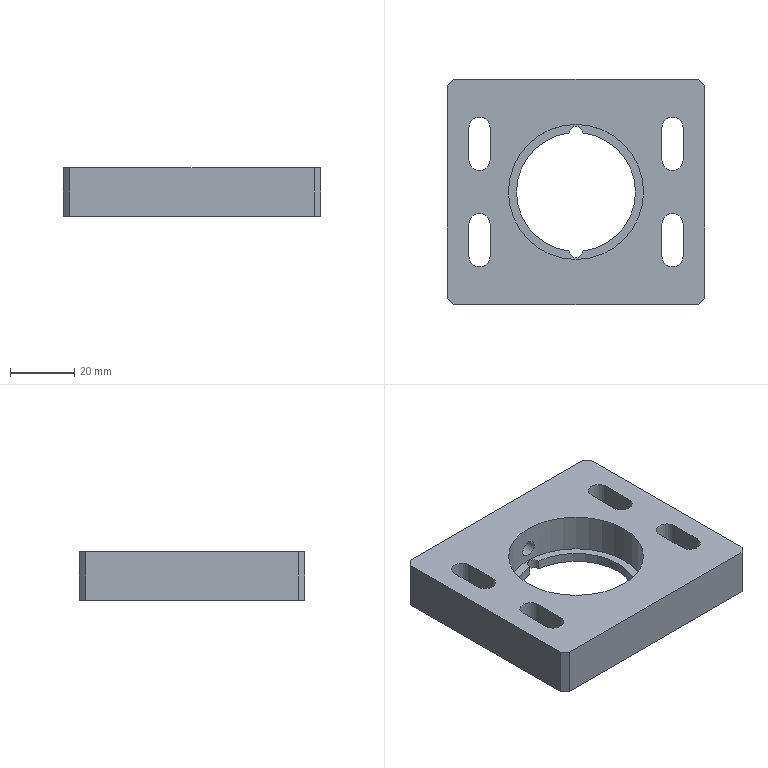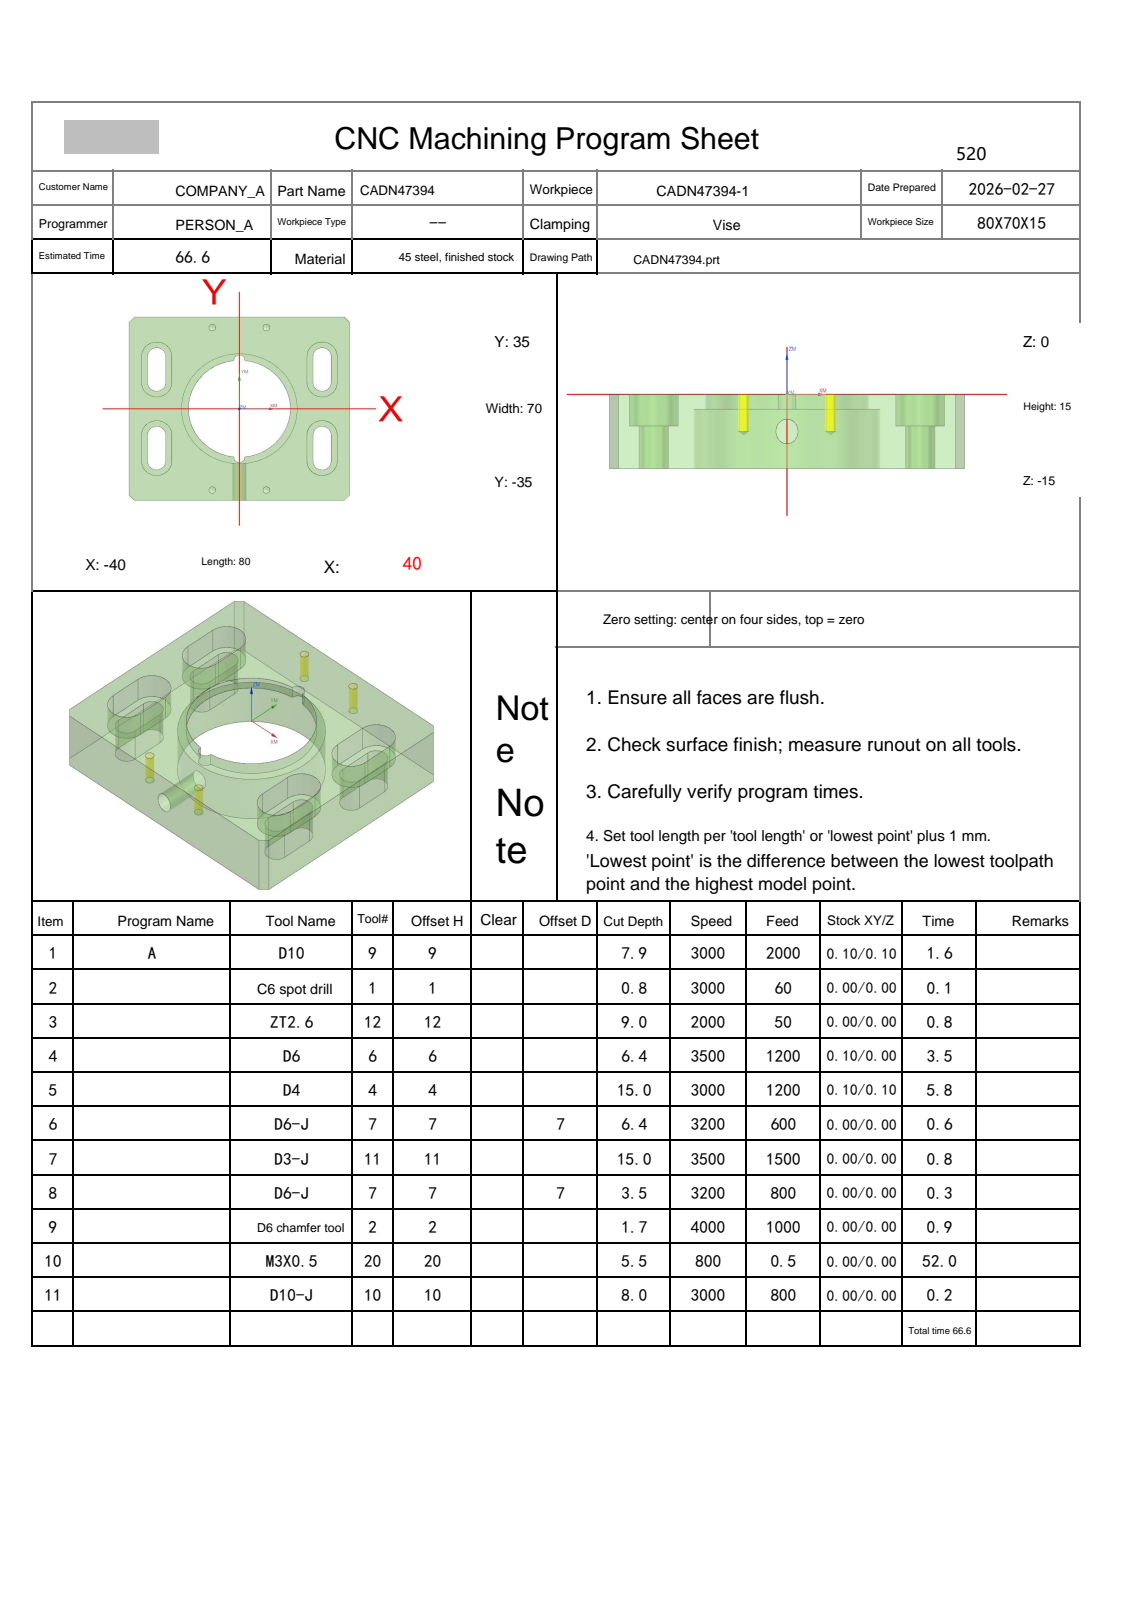NC program | NX | posted by the shop | part box 80 x 70 x 15 mm
Lines 1592 to 3269 of 4817, first 1205 of 1678 lines:
N5 T04 M06
(D4  D=4. R=0. H=04 ce=0.10 di=0.10)
G00 G90 G54 X31.2 Y15. M03 S3000
G43 H04 Z50.
M08
Z-5.9
G01 Y20. Z-5.927 F1200.
G03 X30. Y21.2 Z-5.937 I-1.2 J0.0
X28.8 Y20. Z-5.948 I0.0 J-1.2
G01 Y10. Z-6.002
G03 X30. Y8.8 Z-6.012 I1.2 J0.0
X31.2 Y10. Z-6.022 I0.0 J1.2
G01 Y20. Z-6.076
G03 X30. Y21.2 Z-6.086 I-1.2 J0.0
X28.8 Y20. Z-6.097 I0.0 J-1.2
G01 Y10. Z-6.151
G03 X30. Y8.8 Z-6.161 I1.2 J0.0
X31.2 Y10. Z-6.171 I0.0 J1.2
G01 Y20. Z-6.225
G03 X30. Y21.2 Z-6.236 I-1.2 J0.0
X28.8 Y20. Z-6.246 I0.0 J-1.2
G01 Y10. Z-6.3
G03 X30. Y8.8 Z-6.31 I1.2 J0.0
X31.2 Y10. Z-6.32 I0.0 J1.2
G01 Y20. Z-6.375
G03 X30. Y21.2 Z-6.385 I-1.2 J0.0
X28.8 Y20. Z-6.395 I0.0 J-1.2
G01 Y10. Z-6.449
G03 X30. Y8.8 Z-6.459 I1.2 J0.0
X31.2 Y10. Z-6.47 I0.0 J1.2
G01 Y20. Z-6.524
G03 X30. Y21.2 Z-6.534 I-1.2 J0.0
X28.8 Y20. Z-6.544 I0.0 J-1.2
G01 Y10. Z-6.598
G03 X30. Y8.8 Z-6.609 I1.2 J0.0
X31.2 Y10. Z-6.619 I0.0 J1.2
G01 Y20. Z-6.673
G03 X30. Y21.2 Z-6.683 I-1.2 J0.0
X28.8 Y20. Z-6.693 I0.0 J-1.2
G01 Y10. Z-6.748
G03 X30. Y8.8 Z-6.758 I1.2 J0.0
X31.2 Y10. Z-6.768 I0.0 J1.2
G01 Y20. Z-6.822
G03 X30. Y21.2 Z-6.832 I-1.2 J0.0
X28.8 Y20. Z-6.843 I0.0 J-1.2
G01 Y10. Z-6.897
G03 X30. Y8.8 Z-6.907 I1.2 J0.0
X31.2 Y10. Z-6.917 I0.0 J1.2
G01 Y20. Z-6.971
G03 X30. Y21.2 Z-6.982 I-1.2 J0.0
X28.8 Y20. Z-6.992 I0.0 J-1.2
G01 Y10. Z-7.046
G03 X30. Y8.8 Z-7.056 I1.2 J0.0
X31.2 Y10. Z-7.066 I0.0 J1.2
G01 Y20. Z-7.121
G03 X30. Y21.2 Z-7.131 I-1.2 J0.0
X28.8 Y20. Z-7.141 I0.0 J-1.2
G01 Y10. Z-7.195
G03 X30. Y8.8 Z-7.205 I1.2 J0.0
X31.2 Y10. Z-7.216 I0.0 J1.2
G01 Y20. Z-7.27
G03 X30. Y21.2 Z-7.28 I-1.2 J0.0
X28.8 Y20. Z-7.29 I0.0 J-1.2
G01 Y10. Z-7.344
G03 X30. Y8.8 Z-7.355 I1.2 J0.0
X31.2 Y10. Z-7.365 I0.0 J1.2
G01 Y20. Z-7.419
G03 X30. Y21.2 Z-7.429 I-1.2 J0.0
X28.8 Y20. Z-7.439 I0.0 J-1.2
G01 Y10. Z-7.493
G03 X30. Y8.8 Z-7.504 I1.2 J0.0
X31.2 Y10. Z-7.514 I0.0 J1.2
G01 Y20. Z-7.568
G03 X30. Y21.2 Z-7.578 I-1.2 J0.0
X28.8 Y20. Z-7.588 I0.0 J-1.2
G01 Y10. Z-7.643
G03 X30. Y8.8 Z-7.653 I1.2 J0.0
X31.2 Y10. Z-7.663 I0.0 J1.2
G01 Y20. Z-7.717
G03 X30. Y21.2 Z-7.727 I-1.2 J0.0
X28.8 Y20. Z-7.738 I0.0 J-1.2
G01 Y10. Z-7.792
G03 X30. Y8.8 Z-7.802 I1.2 J0.0
X31.2 Y10. Z-7.812 I0.0 J1.2
G01 Y20. Z-7.866
G03 X30. Y21.2 Z-7.877 I-1.2 J0.0
X28.8 Y20. Z-7.887 I0.0 J-1.2
G01 Y10. Z-7.941
G03 X30. Y8.8 Z-7.951 I1.2 J0.0
X31.2 Y10. Z-7.961 I0.0 J1.2
G01 Y20. Z-8.016
G03 X30. Y21.2 Z-8.026 I-1.2 J0.0
X28.8 Y20. Z-8.036 I0.0 J-1.2
G01 Y10. Z-8.09
G03 X30. Y8.8 Z-8.1 I1.2 J0.0
X31.2 Y10. Z-8.111 I0.0 J1.2
G01 Y20. Z-8.165
G03 X30. Y21.2 Z-8.175 I-1.2 J0.0
X28.8 Y20. Z-8.185 I0.0 J-1.2
G01 Y10. Z-8.239
G03 X30. Y8.8 Z-8.25 I1.2 J0.0
X31.2 Y10. Z-8.26 I0.0 J1.2
G01 Y20. Z-8.314
G03 X30. Y21.2 Z-8.324 I-1.2 J0.0
X28.8 Y20. Z-8.334 I0.0 J-1.2
G01 Y10. Z-8.389
G03 X30. Y8.8 Z-8.399 I1.2 J0.0
X31.2 Y10. Z-8.409 I0.0 J1.2
G01 Y20. Z-8.463
G03 X30. Y21.2 Z-8.473 I-1.2 J0.0
X28.8 Y20. Z-8.484 I0.0 J-1.2
G01 Y10. Z-8.538
G03 X30. Y8.8 Z-8.548 I1.2 J0.0
X31.2 Y10. Z-8.558 I0.0 J1.2
G01 Y20. Z-8.612
G03 X30. Y21.2 Z-8.623 I-1.2 J0.0
X28.8 Y20. Z-8.633 I0.0 J-1.2
G01 Y10. Z-8.687
G03 X30. Y8.8 Z-8.697 I1.2 J0.0
X31.2 Y10. Z-8.707 I0.0 J1.2
G01 Y20. Z-8.762
G03 X30. Y21.2 Z-8.772 I-1.2 J0.0
X28.8 Y20. Z-8.782 I0.0 J-1.2
G01 Y10. Z-8.836
G03 X30. Y8.8 Z-8.846 I1.2 J0.0
X31.2 Y10. Z-8.857 I0.0 J1.2
G01 Y20. Z-8.911
G03 X30. Y21.2 Z-8.921 I-1.2 J0.0
X28.8 Y20. Z-8.931 I0.0 J-1.2
G01 Y10. Z-8.985
G03 X30. Y8.8 Z-8.995 I1.2 J0.0
X31.2 Y10. Z-9.006 I0.0 J1.2
G01 Y20. Z-9.06
G03 X30. Y21.2 Z-9.07 I-1.2 J0.0
X28.8 Y20. Z-9.08 I0.0 J-1.2
G01 Y10. Z-9.134
G03 X30. Y8.8 Z-9.145 I1.2 J0.0
X31.2 Y10. Z-9.155 I0.0 J1.2
G01 Y20. Z-9.209
G03 X30. Y21.2 Z-9.219 I-1.2 J0.0
X28.8 Y20. Z-9.229 I0.0 J-1.2
G01 Y10. Z-9.284
G03 X30. Y8.8 Z-9.294 I1.2 J0.0
X31.2 Y10. Z-9.304 I0.0 J1.2
G01 Y20. Z-9.358
G03 X30. Y21.2 Z-9.368 I-1.2 J0.0
X28.8 Y20. Z-9.379 I0.0 J-1.2
G01 Y10. Z-9.433
G03 X30. Y8.8 Z-9.443 I1.2 J0.0
X31.2 Y10. Z-9.453 I0.0 J1.2
G01 Y20. Z-9.507
G03 X30. Y21.2 Z-9.518 I-1.2 J0.0
X28.8 Y20. Z-9.528 I0.0 J-1.2
G01 Y10. Z-9.582
G03 X30. Y8.8 Z-9.592 I1.2 J0.0
X31.2 Y10. Z-9.602 I0.0 J1.2
G01 Y20. Z-9.657
G03 X30. Y21.2 Z-9.667 I-1.2 J0.0
X28.8 Y20. Z-9.677 I0.0 J-1.2
G01 Y10. Z-9.731
G03 X30. Y8.8 Z-9.741 I1.2 J0.0
X31.2 Y10. Z-9.752 I0.0 J1.2
G01 Y20. Z-9.806
G03 X30. Y21.2 Z-9.816 I-1.2 J0.0
X28.8 Y20. Z-9.826 I0.0 J-1.2
G01 Y10. Z-9.88
G03 X30. Y8.8 Z-9.891 I1.2 J0.0
X31.2 Y10. Z-9.901 I0.0 J1.2
G01 Y20. Z-9.955
G03 X30. Y21.2 Z-9.965 I-1.2 J0.0
X28.8 Y20. Z-9.975 I0.0 J-1.2
G01 Y10. Z-10.03
G03 X30. Y8.8 Z-10.04 I1.2 J0.0
X31.2 Y10. Z-10.05 I0.0 J1.2
G01 Y20. Z-10.104
G03 X30. Y21.2 Z-10.114 I-1.2 J0.0
X28.8 Y20. Z-10.125 I0.0 J-1.2
G01 Y10. Z-10.179
G03 X30. Y8.8 Z-10.189 I1.2 J0.0
X31.2 Y10. Z-10.199 I0.0 J1.2
G01 Y20. Z-10.253
G03 X30. Y21.2 Z-10.264 I-1.2 J0.0
X28.8 Y20. Z-10.274 I0.0 J-1.2
G01 Y10. Z-10.328
G03 X30. Y8.8 Z-10.338 I1.2 J0.0
X31.2 Y10. Z-10.348 I0.0 J1.2
G01 Y20. Z-10.402
G03 X30. Y21.2 Z-10.413 I-1.2 J0.0
X28.8 Y20. Z-10.423 I0.0 J-1.2
G01 Y10. Z-10.477
G03 X30. Y8.8 Z-10.487 I1.2 J0.0
X31.2 Y10. Z-10.498 I0.0 J1.2
G01 Y20. Z-10.552
G03 X30. Y21.2 Z-10.562 I-1.2 J0.0
X28.8 Y20. Z-10.572 I0.0 J-1.2
G01 Y10. Z-10.626
G03 X30. Y8.8 Z-10.636 I1.2 J0.0
X31.2 Y10. Z-10.647 I0.0 J1.2
G01 Y20. Z-10.701
G03 X30. Y21.2 Z-10.711 I-1.2 J0.0
X28.8 Y20. Z-10.721 I0.0 J-1.2
G01 Y10. Z-10.775
G03 X30. Y8.8 Z-10.786 I1.2 J0.0
X31.2 Y10. Z-10.796 I0.0 J1.2
G01 Y20. Z-10.85
G03 X30. Y21.2 Z-10.86 I-1.2 J0.0
X28.8 Y20. Z-10.87 I0.0 J-1.2
G01 Y10. Z-10.925
G03 X30. Y8.8 Z-10.935 I1.2 J0.0
X31.2 Y10. Z-10.945 I0.0 J1.2
G01 Y20. Z-10.999
G03 X30. Y21.2 Z-11.009 I-1.2 J0.0
X28.8 Y20. Z-11.02 I0.0 J-1.2
G01 Y10. Z-11.074
G03 X30. Y8.8 Z-11.084 I1.2 J0.0
X31.2 Y10. Z-11.094 I0.0 J1.2
G01 Y20. Z-11.148
G03 X30. Y21.2 Z-11.159 I-1.2 J0.0
X28.8 Y20. Z-11.169 I0.0 J-1.2
G01 Y10. Z-11.223
G03 X30. Y8.8 Z-11.233 I1.2 J0.0
X31.2 Y10. Z-11.243 I0.0 J1.2
G01 Y20. Z-11.298
G03 X30. Y21.2 Z-11.308 I-1.2 J0.0
X28.8 Y20. Z-11.318 I0.0 J-1.2
G01 Y10. Z-11.372
G03 X30. Y8.8 Z-11.382 I1.2 J0.0
X31.2 Y10. Z-11.393 I0.0 J1.2
G01 Y20. Z-11.447
G03 X30. Y21.2 Z-11.457 I-1.2 J0.0
X28.8 Y20. Z-11.467 I0.0 J-1.2
G01 Y10. Z-11.521
G03 X30. Y8.8 Z-11.532 I1.2 J0.0
X31.2 Y10. Z-11.542 I0.0 J1.2
G01 Y20. Z-11.596
G03 X30. Y21.2 Z-11.606 I-1.2 J0.0
X28.8 Y20. Z-11.616 I0.0 J-1.2
G01 Y10. Z-11.671
G03 X30. Y8.8 Z-11.681 I1.2 J0.0
X31.2 Y10. Z-11.691 I0.0 J1.2
G01 Y20. Z-11.745
G03 X30. Y21.2 Z-11.755 I-1.2 J0.0
X28.8 Y20. Z-11.766 I0.0 J-1.2
G01 Y10. Z-11.82
G03 X30. Y8.8 Z-11.83 I1.2 J0.0
X31.2 Y10. Z-11.84 I0.0 J1.2
G01 Y20. Z-11.894
G03 X30. Y21.2 Z-11.905 I-1.2 J0.0
X28.8 Y20. Z-11.915 I0.0 J-1.2
G01 Y10. Z-11.969
G03 X30. Y8.8 Z-11.979 I1.2 J0.0
X31.2 Y10. Z-11.989 I0.0 J1.2
G01 Y20. Z-12.043
G03 X30. Y21.2 Z-12.054 I-1.2 J0.0
X28.8 Y20. Z-12.064 I0.0 J-1.2
G01 Y10. Z-12.118
G03 X30. Y8.8 Z-12.128 I1.2 J0.0
X31.2 Y10. Z-12.138 I0.0 J1.2
G01 Y20. Z-12.193
G03 X30. Y21.2 Z-12.203 I-1.2 J0.0
X28.8 Y20. Z-12.213 I0.0 J-1.2
G01 Y10. Z-12.267
G03 X30. Y8.8 Z-12.277 I1.2 J0.0
X31.2 Y10. Z-12.288 I0.0 J1.2
G01 Y20. Z-12.342
G03 X30. Y21.2 Z-12.352 I-1.2 J0.0
X28.8 Y20. Z-12.362 I0.0 J-1.2
G01 Y10. Z-12.416
G03 X30. Y8.8 Z-12.427 I1.2 J0.0
X31.2 Y10. Z-12.437 I0.0 J1.2
G01 Y20. Z-12.491
G03 X30. Y21.2 Z-12.501 I-1.2 J0.0
X28.8 Y20. Z-12.511 I0.0 J-1.2
G01 Y10. Z-12.566
G03 X30. Y8.8 Z-12.576 I1.2 J0.0
X31.2 Y10. Z-12.586 I0.0 J1.2
G01 Y20. Z-12.64
G03 X30. Y21.2 Z-12.65 I-1.2 J0.0
X28.8 Y20. Z-12.661 I0.0 J-1.2
G01 Y10. Z-12.715
G03 X30. Y8.8 Z-12.725 I1.2 J0.0
X31.2 Y10. Z-12.735 I0.0 J1.2
G01 Y20. Z-12.789
G03 X30. Y21.2 Z-12.8 I-1.2 J0.0
X28.8 Y20. Z-12.81 I0.0 J-1.2
G01 Y10. Z-12.864
G03 X30. Y8.8 Z-12.874 I1.2 J0.0
X31.2 Y10. Z-12.884 I0.0 J1.2
G01 Y20. Z-12.939
G03 X30. Y21.2 Z-12.949 I-1.2 J0.0
X28.8 Y20. Z-12.959 I0.0 J-1.2
G01 Y10. Z-13.013
G03 X30. Y8.8 Z-13.023 I1.2 J0.0
X31.2 Y10. Z-13.034 I0.0 J1.2
G01 Y20. Z-13.088
G03 X30. Y21.2 Z-13.098 I-1.2 J0.0
X28.8 Y20. Z-13.108 I0.0 J-1.2
G01 Y10. Z-13.162
G03 X30. Y8.8 Z-13.173 I1.2 J0.0
X31.2 Y10. Z-13.183 I0.0 J1.2
G01 Y20. Z-13.237
G03 X30. Y21.2 Z-13.247 I-1.2 J0.0
X28.8 Y20. Z-13.257 I0.0 J-1.2
G01 Y10. Z-13.312
G03 X30. Y8.8 Z-13.322 I1.2 J0.0
X31.2 Y10. Z-13.332 I0.0 J1.2
G01 Y20. Z-13.386
G03 X30. Y21.2 Z-13.396 I-1.2 J0.0
X28.8 Y20. Z-13.407 I0.0 J-1.2
G01 Y10. Z-13.461
G03 X30. Y8.8 Z-13.471 I1.2 J0.0
X31.2 Y10. Z-13.481 I0.0 J1.2
G01 Y20. Z-13.535
G03 X30. Y21.2 Z-13.545 I-1.2 J0.0
X28.8 Y20. Z-13.556 I0.0 J-1.2
G01 Y10. Z-13.61
G03 X30. Y8.8 Z-13.62 I1.2 J0.0
X31.2 Y10. Z-13.63 I0.0 J1.2
G01 Y20. Z-13.684
G03 X30. Y21.2 Z-13.695 I-1.2 J0.0
X28.8 Y20. Z-13.705 I0.0 J-1.2
G01 Y10. Z-13.759
G03 X30. Y8.8 Z-13.769 I1.2 J0.0
X31.2 Y10. Z-13.779 I0.0 J1.2
G01 Y20. Z-13.834
G03 X30. Y21.2 Z-13.844 I-1.2 J0.0
X28.8 Y20. Z-13.854 I0.0 J-1.2
G01 Y10. Z-13.908
G03 X30. Y8.8 Z-13.918 I1.2 J0.0
X31.2 Y10. Z-13.929 I0.0 J1.2
G01 Y20. Z-13.983
G03 X30. Y21.2 Z-13.993 I-1.2 J0.0
X28.8 Y20. Z-14.003 I0.0 J-1.2
G01 Y10. Z-14.057
G03 X30. Y8.8 Z-14.068 I1.2 J0.0
X31.2 Y10. Z-14.078 I0.0 J1.2
G01 Y20. Z-14.132
G03 X30. Y21.2 Z-14.142 I-1.2 J0.0
X28.8 Y20. Z-14.152 I0.0 J-1.2
G01 Y10. Z-14.207
G03 X30. Y8.8 Z-14.217 I1.2 J0.0
X31.2 Y10. Z-14.227 I0.0 J1.2
G01 Y20. Z-14.281
G03 X30. Y21.2 Z-14.291 I-1.2 J0.0
X28.8 Y20. Z-14.302 I0.0 J-1.2
G01 Y10. Z-14.356
G03 X30. Y8.8 Z-14.366 I1.2 J0.0
X31.2 Y10. Z-14.376 I0.0 J1.2
G01 Y20. Z-14.43
G03 X30. Y21.2 Z-14.441 I-1.2 J0.0
X28.8 Y20. Z-14.451 I0.0 J-1.2
G01 Y10. Z-14.505
G03 X30. Y8.8 Z-14.515 I1.2 J0.0
X31.2 Y10. Z-14.525 I0.0 J1.2
G01 Y20. Z-14.58
G03 X30. Y21.2 Z-14.59 I-1.2 J0.0
X28.8 Y20. Z-14.6 I0.0 J-1.2
G01 Y10. Z-14.654
G03 X30. Y8.8 Z-14.664 I1.2 J0.0
X31.2 Y10. Z-14.675 I0.0 J1.2
G01 Y20. Z-14.729
G03 X30. Y21.2 Z-14.739 I-1.2 J0.0
X28.8 Y20. Z-14.749 I0.0 J-1.2
G01 Y10. Z-14.803
G03 X30. Y8.8 Z-14.814 I1.2 J0.0
X31.2 Y10. Z-14.824 I0.0 J1.2
G01 Y20. Z-14.878
G03 X30. Y21.2 Z-14.888 I-1.2 J0.0
X28.8 Y20. Z-14.898 I0.0 J-1.2
G01 Y10. Z-14.952
G03 X30. Y8.8 Z-14.963 I1.2 J0.0
X31.2 Y10. Z-14.973 I0.0 J1.2
G01 Y15. Z-15.
Y20.
G03 X30. Y21.2 I-1.2 J0.0
X28.8 Y20. I0.0 J-1.2
G01 Y10.
G03 X30. Y8.8 I1.2 J0.0
X31.2 Y10. I0.0 J1.2
G01 Y15.
Y15.5
Z-14.
G00 Z50.
Y-15.
Z-5.9
G01 Y-10. Z-5.927
G03 X30. Y-8.8 Z-5.937 I-1.2 J0.0
X28.8 Y-10. Z-5.948 I0.0 J-1.2
G01 Y-20. Z-6.002
G03 X30. Y-21.2 Z-6.012 I1.2 J0.0
X31.2 Y-20. Z-6.022 I0.0 J1.2
G01 Y-10. Z-6.076
G03 X30. Y-8.8 Z-6.086 I-1.2 J0.0
X28.8 Y-10. Z-6.097 I0.0 J-1.2
G01 Y-20. Z-6.151
G03 X30. Y-21.2 Z-6.161 I1.2 J0.0
X31.2 Y-20. Z-6.171 I0.0 J1.2
G01 Y-10. Z-6.225
G03 X30. Y-8.8 Z-6.236 I-1.2 J0.0
X28.8 Y-10. Z-6.246 I0.0 J-1.2
G01 Y-20. Z-6.3
G03 X30. Y-21.2 Z-6.31 I1.2 J0.0
X31.2 Y-20. Z-6.32 I0.0 J1.2
G01 Y-10. Z-6.375
G03 X30. Y-8.8 Z-6.385 I-1.2 J0.0
X28.8 Y-10. Z-6.395 I0.0 J-1.2
G01 Y-20. Z-6.449
G03 X30. Y-21.2 Z-6.459 I1.2 J0.0
X31.2 Y-20. Z-6.47 I0.0 J1.2
G01 Y-10. Z-6.524
G03 X30. Y-8.8 Z-6.534 I-1.2 J0.0
X28.8 Y-10. Z-6.544 I0.0 J-1.2
G01 Y-20. Z-6.598
G03 X30. Y-21.2 Z-6.609 I1.2 J0.0
X31.2 Y-20. Z-6.619 I0.0 J1.2
G01 Y-10. Z-6.673
G03 X30. Y-8.8 Z-6.683 I-1.2 J0.0
X28.8 Y-10. Z-6.693 I0.0 J-1.2
G01 Y-20. Z-6.748
G03 X30. Y-21.2 Z-6.758 I1.2 J0.0
X31.2 Y-20. Z-6.768 I0.0 J1.2
G01 Y-10. Z-6.822
G03 X30. Y-8.8 Z-6.832 I-1.2 J0.0
X28.8 Y-10. Z-6.843 I0.0 J-1.2
G01 Y-20. Z-6.897
G03 X30. Y-21.2 Z-6.907 I1.2 J0.0
X31.2 Y-20. Z-6.917 I0.0 J1.2
G01 Y-10. Z-6.971
G03 X30. Y-8.8 Z-6.982 I-1.2 J0.0
X28.8 Y-10. Z-6.992 I0.0 J-1.2
G01 Y-20. Z-7.046
G03 X30. Y-21.2 Z-7.056 I1.2 J0.0
X31.2 Y-20. Z-7.066 I0.0 J1.2
G01 Y-10. Z-7.121
G03 X30. Y-8.8 Z-7.131 I-1.2 J0.0
X28.8 Y-10. Z-7.141 I0.0 J-1.2
G01 Y-20. Z-7.195
G03 X30. Y-21.2 Z-7.205 I1.2 J0.0
X31.2 Y-20. Z-7.216 I0.0 J1.2
G01 Y-10. Z-7.27
G03 X30. Y-8.8 Z-7.28 I-1.2 J0.0
X28.8 Y-10. Z-7.29 I0.0 J-1.2
G01 Y-20. Z-7.344
G03 X30. Y-21.2 Z-7.355 I1.2 J0.0
X31.2 Y-20. Z-7.365 I0.0 J1.2
G01 Y-10. Z-7.419
G03 X30. Y-8.8 Z-7.429 I-1.2 J0.0
X28.8 Y-10. Z-7.439 I0.0 J-1.2
G01 Y-20. Z-7.493
G03 X30. Y-21.2 Z-7.504 I1.2 J0.0
X31.2 Y-20. Z-7.514 I0.0 J1.2
G01 Y-10. Z-7.568
G03 X30. Y-8.8 Z-7.578 I-1.2 J0.0
X28.8 Y-10. Z-7.588 I0.0 J-1.2
G01 Y-20. Z-7.643
G03 X30. Y-21.2 Z-7.653 I1.2 J0.0
X31.2 Y-20. Z-7.663 I0.0 J1.2
G01 Y-10. Z-7.717
G03 X30. Y-8.8 Z-7.727 I-1.2 J0.0
X28.8 Y-10. Z-7.738 I0.0 J-1.2
G01 Y-20. Z-7.792
G03 X30. Y-21.2 Z-7.802 I1.2 J0.0
X31.2 Y-20. Z-7.812 I0.0 J1.2
G01 Y-10. Z-7.866
G03 X30. Y-8.8 Z-7.877 I-1.2 J0.0
X28.8 Y-10. Z-7.887 I0.0 J-1.2
G01 Y-20. Z-7.941
G03 X30. Y-21.2 Z-7.951 I1.2 J0.0
X31.2 Y-20. Z-7.961 I0.0 J1.2
G01 Y-10. Z-8.016
G03 X30. Y-8.8 Z-8.026 I-1.2 J0.0
X28.8 Y-10. Z-8.036 I0.0 J-1.2
G01 Y-20. Z-8.09
G03 X30. Y-21.2 Z-8.1 I1.2 J0.0
X31.2 Y-20. Z-8.111 I0.0 J1.2
G01 Y-10. Z-8.165
G03 X30. Y-8.8 Z-8.175 I-1.2 J0.0
X28.8 Y-10. Z-8.185 I0.0 J-1.2
G01 Y-20. Z-8.239
G03 X30. Y-21.2 Z-8.25 I1.2 J0.0
X31.2 Y-20. Z-8.26 I0.0 J1.2
G01 Y-10. Z-8.314
G03 X30. Y-8.8 Z-8.324 I-1.2 J0.0
X28.8 Y-10. Z-8.334 I0.0 J-1.2
G01 Y-20. Z-8.389
G03 X30. Y-21.2 Z-8.399 I1.2 J0.0
X31.2 Y-20. Z-8.409 I0.0 J1.2
G01 Y-10. Z-8.463
G03 X30. Y-8.8 Z-8.473 I-1.2 J0.0
X28.8 Y-10. Z-8.484 I0.0 J-1.2
G01 Y-20. Z-8.538
G03 X30. Y-21.2 Z-8.548 I1.2 J0.0
X31.2 Y-20. Z-8.558 I0.0 J1.2
G01 Y-10. Z-8.612
G03 X30. Y-8.8 Z-8.623 I-1.2 J0.0
X28.8 Y-10. Z-8.633 I0.0 J-1.2
G01 Y-20. Z-8.687
G03 X30. Y-21.2 Z-8.697 I1.2 J0.0
X31.2 Y-20. Z-8.707 I0.0 J1.2
G01 Y-10. Z-8.762
G03 X30. Y-8.8 Z-8.772 I-1.2 J0.0
X28.8 Y-10. Z-8.782 I0.0 J-1.2
G01 Y-20. Z-8.836
G03 X30. Y-21.2 Z-8.846 I1.2 J0.0
X31.2 Y-20. Z-8.857 I0.0 J1.2
G01 Y-10. Z-8.911
G03 X30. Y-8.8 Z-8.921 I-1.2 J0.0
X28.8 Y-10. Z-8.931 I0.0 J-1.2
G01 Y-20. Z-8.985
G03 X30. Y-21.2 Z-8.995 I1.2 J0.0
X31.2 Y-20. Z-9.006 I0.0 J1.2
G01 Y-10. Z-9.06
G03 X30. Y-8.8 Z-9.07 I-1.2 J0.0
X28.8 Y-10. Z-9.08 I0.0 J-1.2
G01 Y-20. Z-9.134
G03 X30. Y-21.2 Z-9.145 I1.2 J0.0
X31.2 Y-20. Z-9.155 I0.0 J1.2
G01 Y-10. Z-9.209
G03 X30. Y-8.8 Z-9.219 I-1.2 J0.0
X28.8 Y-10. Z-9.229 I0.0 J-1.2
G01 Y-20. Z-9.284
G03 X30. Y-21.2 Z-9.294 I1.2 J0.0
X31.2 Y-20. Z-9.304 I0.0 J1.2
G01 Y-10. Z-9.358
G03 X30. Y-8.8 Z-9.368 I-1.2 J0.0
X28.8 Y-10. Z-9.379 I0.0 J-1.2
G01 Y-20. Z-9.433
G03 X30. Y-21.2 Z-9.443 I1.2 J0.0
X31.2 Y-20. Z-9.453 I0.0 J1.2
G01 Y-10. Z-9.507
G03 X30. Y-8.8 Z-9.518 I-1.2 J0.0
X28.8 Y-10. Z-9.528 I0.0 J-1.2
G01 Y-20. Z-9.582
G03 X30. Y-21.2 Z-9.592 I1.2 J0.0
X31.2 Y-20. Z-9.602 I0.0 J1.2
G01 Y-10. Z-9.657
G03 X30. Y-8.8 Z-9.667 I-1.2 J0.0
X28.8 Y-10. Z-9.677 I0.0 J-1.2
G01 Y-20. Z-9.731
G03 X30. Y-21.2 Z-9.741 I1.2 J0.0
X31.2 Y-20. Z-9.752 I0.0 J1.2
G01 Y-10. Z-9.806
G03 X30. Y-8.8 Z-9.816 I-1.2 J0.0
X28.8 Y-10. Z-9.826 I0.0 J-1.2
G01 Y-20. Z-9.88
G03 X30. Y-21.2 Z-9.891 I1.2 J0.0
X31.2 Y-20. Z-9.901 I0.0 J1.2
G01 Y-10. Z-9.955
G03 X30. Y-8.8 Z-9.965 I-1.2 J0.0
X28.8 Y-10. Z-9.975 I0.0 J-1.2
G01 Y-20. Z-10.03
G03 X30. Y-21.2 Z-10.04 I1.2 J0.0
X31.2 Y-20. Z-10.05 I0.0 J1.2
G01 Y-10. Z-10.104
G03 X30. Y-8.8 Z-10.114 I-1.2 J0.0
X28.8 Y-10. Z-10.125 I0.0 J-1.2
G01 Y-20. Z-10.179
G03 X30. Y-21.2 Z-10.189 I1.2 J0.0
X31.2 Y-20. Z-10.199 I0.0 J1.2
G01 Y-10. Z-10.253
G03 X30. Y-8.8 Z-10.264 I-1.2 J0.0
X28.8 Y-10. Z-10.274 I0.0 J-1.2
G01 Y-20. Z-10.328
G03 X30. Y-21.2 Z-10.338 I1.2 J0.0
X31.2 Y-20. Z-10.348 I0.0 J1.2
G01 Y-10. Z-10.402
G03 X30. Y-8.8 Z-10.413 I-1.2 J0.0
X28.8 Y-10. Z-10.423 I0.0 J-1.2
G01 Y-20. Z-10.477
G03 X30. Y-21.2 Z-10.487 I1.2 J0.0
X31.2 Y-20. Z-10.498 I0.0 J1.2
G01 Y-10. Z-10.552
G03 X30. Y-8.8 Z-10.562 I-1.2 J0.0
X28.8 Y-10. Z-10.572 I0.0 J-1.2
G01 Y-20. Z-10.626
G03 X30. Y-21.2 Z-10.636 I1.2 J0.0
X31.2 Y-20. Z-10.647 I0.0 J1.2
G01 Y-10. Z-10.701
G03 X30. Y-8.8 Z-10.711 I-1.2 J0.0
X28.8 Y-10. Z-10.721 I0.0 J-1.2
G01 Y-20. Z-10.775
G03 X30. Y-21.2 Z-10.786 I1.2 J0.0
X31.2 Y-20. Z-10.796 I0.0 J1.2
G01 Y-10. Z-10.85
G03 X30. Y-8.8 Z-10.86 I-1.2 J0.0
X28.8 Y-10. Z-10.87 I0.0 J-1.2
G01 Y-20. Z-10.925
G03 X30. Y-21.2 Z-10.935 I1.2 J0.0
X31.2 Y-20. Z-10.945 I0.0 J1.2
G01 Y-10. Z-10.999
G03 X30. Y-8.8 Z-11.009 I-1.2 J0.0
X28.8 Y-10. Z-11.02 I0.0 J-1.2
G01 Y-20. Z-11.074
G03 X30. Y-21.2 Z-11.084 I1.2 J0.0
X31.2 Y-20. Z-11.094 I0.0 J1.2
G01 Y-10. Z-11.148
G03 X30. Y-8.8 Z-11.159 I-1.2 J0.0
X28.8 Y-10. Z-11.169 I0.0 J-1.2
G01 Y-20. Z-11.223
G03 X30. Y-21.2 Z-11.233 I1.2 J0.0
X31.2 Y-20. Z-11.243 I0.0 J1.2
G01 Y-10. Z-11.298
G03 X30. Y-8.8 Z-11.308 I-1.2 J0.0
X28.8 Y-10. Z-11.318 I0.0 J-1.2
G01 Y-20. Z-11.372
G03 X30. Y-21.2 Z-11.382 I1.2 J0.0
X31.2 Y-20. Z-11.393 I0.0 J1.2
G01 Y-10. Z-11.447
G03 X30. Y-8.8 Z-11.457 I-1.2 J0.0
X28.8 Y-10. Z-11.467 I0.0 J-1.2
G01 Y-20. Z-11.521
G03 X30. Y-21.2 Z-11.532 I1.2 J0.0
X31.2 Y-20. Z-11.542 I0.0 J1.2
G01 Y-10. Z-11.596
G03 X30. Y-8.8 Z-11.606 I-1.2 J0.0
X28.8 Y-10. Z-11.616 I0.0 J-1.2
G01 Y-20. Z-11.671
G03 X30. Y-21.2 Z-11.681 I1.2 J0.0
X31.2 Y-20. Z-11.691 I0.0 J1.2
G01 Y-10. Z-11.745
G03 X30. Y-8.8 Z-11.755 I-1.2 J0.0
X28.8 Y-10. Z-11.766 I0.0 J-1.2
G01 Y-20. Z-11.82
G03 X30. Y-21.2 Z-11.83 I1.2 J0.0
X31.2 Y-20. Z-11.84 I0.0 J1.2
G01 Y-10. Z-11.894
G03 X30. Y-8.8 Z-11.905 I-1.2 J0.0
X28.8 Y-10. Z-11.915 I0.0 J-1.2
G01 Y-20. Z-11.969
G03 X30. Y-21.2 Z-11.979 I1.2 J0.0
X31.2 Y-20. Z-11.989 I0.0 J1.2
G01 Y-10. Z-12.043
G03 X30. Y-8.8 Z-12.054 I-1.2 J0.0
X28.8 Y-10. Z-12.064 I0.0 J-1.2
G01 Y-20. Z-12.118
G03 X30. Y-21.2 Z-12.128 I1.2 J0.0
X31.2 Y-20. Z-12.138 I0.0 J1.2
G01 Y-10. Z-12.193
G03 X30. Y-8.8 Z-12.203 I-1.2 J0.0
X28.8 Y-10. Z-12.213 I0.0 J-1.2
G01 Y-20. Z-12.267
G03 X30. Y-21.2 Z-12.277 I1.2 J0.0
X31.2 Y-20. Z-12.288 I0.0 J1.2
G01 Y-10. Z-12.342
G03 X30. Y-8.8 Z-12.352 I-1.2 J0.0
X28.8 Y-10. Z-12.362 I0.0 J-1.2
G01 Y-20. Z-12.416
G03 X30. Y-21.2 Z-12.427 I1.2 J0.0
X31.2 Y-20. Z-12.437 I0.0 J1.2
G01 Y-10. Z-12.491
G03 X30. Y-8.8 Z-12.501 I-1.2 J0.0
X28.8 Y-10. Z-12.511 I0.0 J-1.2
G01 Y-20. Z-12.566
G03 X30. Y-21.2 Z-12.576 I1.2 J0.0
X31.2 Y-20. Z-12.586 I0.0 J1.2
G01 Y-10. Z-12.64
G03 X30. Y-8.8 Z-12.65 I-1.2 J0.0
X28.8 Y-10. Z-12.661 I0.0 J-1.2
G01 Y-20. Z-12.715
G03 X30. Y-21.2 Z-12.725 I1.2 J0.0
X31.2 Y-20. Z-12.735 I0.0 J1.2
G01 Y-10. Z-12.789
G03 X30. Y-8.8 Z-12.8 I-1.2 J0.0
X28.8 Y-10. Z-12.81 I0.0 J-1.2
G01 Y-20. Z-12.864
G03 X30. Y-21.2 Z-12.874 I1.2 J0.0
X31.2 Y-20. Z-12.884 I0.0 J1.2
G01 Y-10. Z-12.939
G03 X30. Y-8.8 Z-12.949 I-1.2 J0.0
X28.8 Y-10. Z-12.959 I0.0 J-1.2
G01 Y-20. Z-13.013
G03 X30. Y-21.2 Z-13.023 I1.2 J0.0
X31.2 Y-20. Z-13.034 I0.0 J1.2
G01 Y-10. Z-13.088
G03 X30. Y-8.8 Z-13.098 I-1.2 J0.0
X28.8 Y-10. Z-13.108 I0.0 J-1.2
G01 Y-20. Z-13.162
G03 X30. Y-21.2 Z-13.173 I1.2 J0.0
X31.2 Y-20. Z-13.183 I0.0 J1.2
G01 Y-10. Z-13.237
G03 X30. Y-8.8 Z-13.247 I-1.2 J0.0
X28.8 Y-10. Z-13.257 I0.0 J-1.2
G01 Y-20. Z-13.312
G03 X30. Y-21.2 Z-13.322 I1.2 J0.0
X31.2 Y-20. Z-13.332 I0.0 J1.2
G01 Y-10. Z-13.386
G03 X30. Y-8.8 Z-13.396 I-1.2 J0.0
X28.8 Y-10. Z-13.407 I0.0 J-1.2
G01 Y-20. Z-13.461
G03 X30. Y-21.2 Z-13.471 I1.2 J0.0
X31.2 Y-20. Z-13.481 I0.0 J1.2
G01 Y-10. Z-13.535
G03 X30. Y-8.8 Z-13.545 I-1.2 J0.0
X28.8 Y-10. Z-13.556 I0.0 J-1.2
G01 Y-20. Z-13.61
G03 X30. Y-21.2 Z-13.62 I1.2 J0.0
X31.2 Y-20. Z-13.63 I0.0 J1.2
G01 Y-10. Z-13.684
G03 X30. Y-8.8 Z-13.695 I-1.2 J0.0
X28.8 Y-10. Z-13.705 I0.0 J-1.2
G01 Y-20. Z-13.759
G03 X30. Y-21.2 Z-13.769 I1.2 J0.0
X31.2 Y-20. Z-13.779 I0.0 J1.2
G01 Y-10. Z-13.834
G03 X30. Y-8.8 Z-13.844 I-1.2 J0.0
X28.8 Y-10. Z-13.854 I0.0 J-1.2
G01 Y-20. Z-13.908
G03 X30. Y-21.2 Z-13.918 I1.2 J0.0
X31.2 Y-20. Z-13.929 I0.0 J1.2
G01 Y-10. Z-13.983
G03 X30. Y-8.8 Z-13.993 I-1.2 J0.0
X28.8 Y-10. Z-14.003 I0.0 J-1.2
G01 Y-20. Z-14.057
G03 X30. Y-21.2 Z-14.068 I1.2 J0.0
X31.2 Y-20. Z-14.078 I0.0 J1.2
G01 Y-10. Z-14.132
G03 X30. Y-8.8 Z-14.142 I-1.2 J0.0
X28.8 Y-10. Z-14.152 I0.0 J-1.2
G01 Y-20. Z-14.207
G03 X30. Y-21.2 Z-14.217 I1.2 J0.0
X31.2 Y-20. Z-14.227 I0.0 J1.2
G01 Y-10. Z-14.281
G03 X30. Y-8.8 Z-14.291 I-1.2 J0.0
X28.8 Y-10. Z-14.302 I0.0 J-1.2
G01 Y-20. Z-14.356
G03 X30. Y-21.2 Z-14.366 I1.2 J0.0
X31.2 Y-20. Z-14.376 I0.0 J1.2
G01 Y-10. Z-14.43
G03 X30. Y-8.8 Z-14.441 I-1.2 J0.0
X28.8 Y-10. Z-14.451 I0.0 J-1.2
G01 Y-20. Z-14.505
G03 X30. Y-21.2 Z-14.515 I1.2 J0.0
X31.2 Y-20. Z-14.525 I0.0 J1.2
G01 Y-10. Z-14.58
G03 X30. Y-8.8 Z-14.59 I-1.2 J0.0
X28.8 Y-10. Z-14.6 I0.0 J-1.2
G01 Y-20. Z-14.654
G03 X30. Y-21.2 Z-14.664 I1.2 J0.0
X31.2 Y-20. Z-14.675 I0.0 J1.2
G01 Y-10. Z-14.729
G03 X30. Y-8.8 Z-14.739 I-1.2 J0.0
X28.8 Y-10. Z-14.749 I0.0 J-1.2
G01 Y-20. Z-14.803
G03 X30. Y-21.2 Z-14.814 I1.2 J0.0
X31.2 Y-20. Z-14.824 I0.0 J1.2
G01 Y-10. Z-14.878
G03 X30. Y-8.8 Z-14.888 I-1.2 J0.0
X28.8 Y-10. Z-14.898 I0.0 J-1.2
G01 Y-20. Z-14.952
G03 X30. Y-21.2 Z-14.963 I1.2 J0.0
X31.2 Y-20. Z-14.973 I0.0 J1.2
G01 Y-15. Z-15.
Y-10.
G03 X30. Y-8.8 I-1.2 J0.0
X28.8 Y-10. I0.0 J-1.2
G01 Y-20.
G03 X30. Y-21.2 I1.2 J0.0
X31.2 Y-20. I0.0 J1.2
G01 Y-15.
Y-14.5
Z-14.
G00 Z50.
X-31.2 Y-15.
Z-5.9
G01 Y-20. Z-5.927
G03 X-30. Y-21.2 Z-5.937 I1.2 J0.0
X-28.8 Y-20. Z-5.948 I0.0 J1.2
G01 Y-10. Z-6.002
G03 X-30. Y-8.8 Z-6.012 I-1.2 J0.0
X-31.2 Y-10. Z-6.022 I0.0 J-1.2
G01 Y-20. Z-6.076
G03 X-30. Y-21.2 Z-6.086 I1.2 J0.0
X-28.8 Y-20. Z-6.097 I0.0 J1.2
G01 Y-10. Z-6.151
G03 X-30. Y-8.8 Z-6.161 I-1.2 J0.0
X-31.2 Y-10. Z-6.171 I0.0 J-1.2
G01 Y-20. Z-6.225
G03 X-30. Y-21.2 Z-6.236 I1.2 J0.0
X-28.8 Y-20. Z-6.246 I0.0 J1.2
G01 Y-10. Z-6.3
G03 X-30. Y-8.8 Z-6.31 I-1.2 J0.0
X-31.2 Y-10. Z-6.32 I0.0 J-1.2
G01 Y-20. Z-6.375
G03 X-30. Y-21.2 Z-6.385 I1.2 J0.0
X-28.8 Y-20. Z-6.395 I0.0 J1.2
G01 Y-10. Z-6.449
G03 X-30. Y-8.8 Z-6.459 I-1.2 J0.0
X-31.2 Y-10. Z-6.47 I0.0 J-1.2
G01 Y-20. Z-6.524
G03 X-30. Y-21.2 Z-6.534 I1.2 J0.0
X-28.8 Y-20. Z-6.544 I0.0 J1.2
G01 Y-10. Z-6.598
G03 X-30. Y-8.8 Z-6.609 I-1.2 J0.0
X-31.2 Y-10. Z-6.619 I0.0 J-1.2
G01 Y-20. Z-6.673
G03 X-30. Y-21.2 Z-6.683 I1.2 J0.0
X-28.8 Y-20. Z-6.693 I0.0 J1.2
G01 Y-10. Z-6.748
G03 X-30. Y-8.8 Z-6.758 I-1.2 J0.0
X-31.2 Y-10. Z-6.768 I0.0 J-1.2
G01 Y-20. Z-6.822
G03 X-30. Y-21.2 Z-6.832 I1.2 J0.0
X-28.8 Y-20. Z-6.843 I0.0 J1.2
G01 Y-10. Z-6.897
G03 X-30. Y-8.8 Z-6.907 I-1.2 J0.0
X-31.2 Y-10. Z-6.917 I0.0 J-1.2
G01 Y-20. Z-6.971
G03 X-30. Y-21.2 Z-6.982 I1.2 J0.0
X-28.8 Y-20. Z-6.992 I0.0 J1.2
G01 Y-10. Z-7.046
G03 X-30. Y-8.8 Z-7.056 I-1.2 J0.0
X-31.2 Y-10. Z-7.066 I0.0 J-1.2
G01 Y-20. Z-7.121
G03 X-30. Y-21.2 Z-7.131 I1.2 J0.0
X-28.8 Y-20. Z-7.141 I0.0 J1.2
G01 Y-10. Z-7.195
G03 X-30. Y-8.8 Z-7.205 I-1.2 J0.0
X-31.2 Y-10. Z-7.216 I0.0 J-1.2
G01 Y-20. Z-7.27
G03 X-30. Y-21.2 Z-7.28 I1.2 J0.0
X-28.8 Y-20. Z-7.29 I0.0 J1.2
G01 Y-10. Z-7.344
G03 X-30. Y-8.8 Z-7.355 I-1.2 J0.0
X-31.2 Y-10. Z-7.365 I0.0 J-1.2
G01 Y-20. Z-7.419
G03 X-30. Y-21.2 Z-7.429 I1.2 J0.0
X-28.8 Y-20. Z-7.439 I0.0 J1.2
G01 Y-10. Z-7.493
G03 X-30. Y-8.8 Z-7.504 I-1.2 J0.0
X-31.2 Y-10. Z-7.514 I0.0 J-1.2
G01 Y-20. Z-7.568
G03 X-30. Y-21.2 Z-7.578 I1.2 J0.0
X-28.8 Y-20. Z-7.588 I0.0 J1.2
G01 Y-10. Z-7.643
G03 X-30. Y-8.8 Z-7.653 I-1.2 J0.0
X-31.2 Y-10. Z-7.663 I0.0 J-1.2
G01 Y-20. Z-7.717
G03 X-30. Y-21.2 Z-7.727 I1.2 J0.0
X-28.8 Y-20. Z-7.738 I0.0 J1.2
G01 Y-10. Z-7.792
G03 X-30. Y-8.8 Z-7.802 I-1.2 J0.0
X-31.2 Y-10. Z-7.812 I0.0 J-1.2
G01 Y-20. Z-7.866
G03 X-30. Y-21.2 Z-7.877 I1.2 J0.0
X-28.8 Y-20. Z-7.887 I0.0 J1.2
G01 Y-10. Z-7.941
G03 X-30. Y-8.8 Z-7.951 I-1.2 J0.0
X-31.2 Y-10. Z-7.961 I0.0 J-1.2
G01 Y-20. Z-8.016
G03 X-30. Y-21.2 Z-8.026 I1.2 J0.0
X-28.8 Y-20. Z-8.036 I0.0 J1.2
G01 Y-10. Z-8.09
G03 X-30. Y-8.8 Z-8.1 I-1.2 J0.0
X-31.2 Y-10. Z-8.111 I0.0 J-1.2
G01 Y-20. Z-8.165
G03 X-30. Y-21.2 Z-8.175 I1.2 J0.0
X-28.8 Y-20. Z-8.185 I0.0 J1.2
G01 Y-10. Z-8.239
G03 X-30. Y-8.8 Z-8.25 I-1.2 J0.0
X-31.2 Y-10. Z-8.26 I0.0 J-1.2
G01 Y-20. Z-8.314
G03 X-30. Y-21.2 Z-8.324 I1.2 J0.0
X-28.8 Y-20. Z-8.334 I0.0 J1.2
G01 Y-10. Z-8.389
G03 X-30. Y-8.8 Z-8.399 I-1.2 J0.0
X-31.2 Y-10. Z-8.409 I0.0 J-1.2
G01 Y-20. Z-8.463
G03 X-30. Y-21.2 Z-8.473 I1.2 J0.0
X-28.8 Y-20. Z-8.484 I0.0 J1.2
G01 Y-10. Z-8.538
G03 X-30. Y-8.8 Z-8.548 I-1.2 J0.0
X-31.2 Y-10. Z-8.558 I0.0 J-1.2
G01 Y-20. Z-8.612
G03 X-30. Y-21.2 Z-8.623 I1.2 J0.0
X-28.8 Y-20. Z-8.633 I0.0 J1.2
G01 Y-10. Z-8.687
G03 X-30. Y-8.8 Z-8.697 I-1.2 J0.0
X-31.2 Y-10. Z-8.707 I0.0 J-1.2
G01 Y-20. Z-8.762
G03 X-30. Y-21.2 Z-8.772 I1.2 J0.0
X-28.8 Y-20. Z-8.782 I0.0 J1.2
G01 Y-10. Z-8.836
G03 X-30. Y-8.8 Z-8.846 I-1.2 J0.0
X-31.2 Y-10. Z-8.857 I0.0 J-1.2
G01 Y-20. Z-8.911
G03 X-30. Y-21.2 Z-8.921 I1.2 J0.0
X-28.8 Y-20. Z-8.931 I0.0 J1.2
G01 Y-10. Z-8.985
G03 X-30. Y-8.8 Z-8.995 I-1.2 J0.0
X-31.2 Y-10. Z-9.006 I0.0 J-1.2
G01 Y-20. Z-9.06
G03 X-30. Y-21.2 Z-9.07 I1.2 J0.0
X-28.8 Y-20. Z-9.08 I0.0 J1.2
G01 Y-10. Z-9.134
G03 X-30. Y-8.8 Z-9.145 I-1.2 J0.0
X-31.2 Y-10. Z-9.155 I0.0 J-1.2
G01 Y-20. Z-9.209
G03 X-30. Y-21.2 Z-9.219 I1.2 J0.0
X-28.8 Y-20. Z-9.229 I0.0 J1.2
G01 Y-10. Z-9.284
G03 X-30. Y-8.8 Z-9.294 I-1.2 J0.0
X-31.2 Y-10. Z-9.304 I0.0 J-1.2
G01 Y-20. Z-9.358
G03 X-30. Y-21.2 Z-9.368 I1.2 J0.0
X-28.8 Y-20. Z-9.379 I0.0 J1.2
G01 Y-10. Z-9.433
G03 X-30. Y-8.8 Z-9.443 I-1.2 J0.0
X-31.2 Y-10. Z-9.453 I0.0 J-1.2
G01 Y-20. Z-9.507
G03 X-30. Y-21.2 Z-9.518 I1.2 J0.0
X-28.8 Y-20. Z-9.528 I0.0 J1.2
G01 Y-10. Z-9.582
G03 X-30. Y-8.8 Z-9.592 I-1.2 J0.0
X-31.2 Y-10. Z-9.602 I0.0 J-1.2
G01 Y-20. Z-9.657
G03 X-30. Y-21.2 Z-9.667 I1.2 J0.0
X-28.8 Y-20. Z-9.677 I0.0 J1.2
G01 Y-10. Z-9.731
G03 X-30. Y-8.8 Z-9.741 I-1.2 J0.0
X-31.2 Y-10. Z-9.752 I0.0 J-1.2
G01 Y-20. Z-9.806
G03 X-30. Y-21.2 Z-9.816 I1.2 J0.0
X-28.8 Y-20. Z-9.826 I0.0 J1.2
G01 Y-10. Z-9.88
G03 X-30. Y-8.8 Z-9.891 I-1.2 J0.0
X-31.2 Y-10. Z-9.901 I0.0 J-1.2
G01 Y-20. Z-9.955
G03 X-30. Y-21.2 Z-9.965 I1.2 J0.0
X-28.8 Y-20. Z-9.975 I0.0 J1.2
G01 Y-10. Z-10.03
G03 X-30. Y-8.8 Z-10.04 I-1.2 J0.0
X-31.2 Y-10. Z-10.05 I0.0 J-1.2
G01 Y-20. Z-10.104
G03 X-30. Y-21.2 Z-10.114 I1.2 J0.0
X-28.8 Y-20. Z-10.125 I0.0 J1.2
G01 Y-10. Z-10.179
G03 X-30. Y-8.8 Z-10.189 I-1.2 J0.0
X-31.2 Y-10. Z-10.199 I0.0 J-1.2
G01 Y-20. Z-10.253
G03 X-30. Y-21.2 Z-10.264 I1.2 J0.0
X-28.8 Y-20. Z-10.274 I0.0 J1.2
G01 Y-10. Z-10.328
G03 X-30. Y-8.8 Z-10.338 I-1.2 J0.0
X-31.2 Y-10. Z-10.348 I0.0 J-1.2
G01 Y-20. Z-10.402
G03 X-30. Y-21.2 Z-10.413 I1.2 J0.0
X-28.8 Y-20. Z-10.423 I0.0 J1.2
G01 Y-10. Z-10.477
G03 X-30. Y-8.8 Z-10.487 I-1.2 J0.0
X-31.2 Y-10. Z-10.498 I0.0 J-1.2
G01 Y-20. Z-10.552
G03 X-30. Y-21.2 Z-10.562 I1.2 J0.0
X-28.8 Y-20. Z-10.572 I0.0 J1.2
G01 Y-10. Z-10.626
G03 X-30. Y-8.8 Z-10.636 I-1.2 J0.0
X-31.2 Y-10. Z-10.647 I0.0 J-1.2
G01 Y-20. Z-10.701
G03 X-30. Y-21.2 Z-10.711 I1.2 J0.0
X-28.8 Y-20. Z-10.721 I0.0 J1.2
G01 Y-10. Z-10.775
G03 X-30. Y-8.8 Z-10.786 I-1.2 J0.0
X-31.2 Y-10. Z-10.796 I0.0 J-1.2
G01 Y-20. Z-10.85
G03 X-30. Y-21.2 Z-10.86 I1.2 J0.0
X-28.8 Y-20. Z-10.87 I0.0 J1.2
G01 Y-10. Z-10.925
G03 X-30. Y-8.8 Z-10.935 I-1.2 J0.0
X-31.2 Y-10. Z-10.945 I0.0 J-1.2
G01 Y-20. Z-10.999
G03 X-30. Y-21.2 Z-11.009 I1.2 J0.0
X-28.8 Y-20. Z-11.02 I0.0 J1.2
G01 Y-10. Z-11.074
G03 X-30. Y-8.8 Z-11.084 I-1.2 J0.0
X-31.2 Y-10. Z-11.094 I0.0 J-1.2
G01 Y-20. Z-11.148
G03 X-30. Y-21.2 Z-11.159 I1.2 J0.0
X-28.8 Y-20. Z-11.169 I0.0 J1.2
G01 Y-10. Z-11.223
G03 X-30. Y-8.8 Z-11.233 I-1.2 J0.0
X-31.2 Y-10. Z-11.243 I0.0 J-1.2
G01 Y-20. Z-11.298
G03 X-30. Y-21.2 Z-11.308 I1.2 J0.0
X-28.8 Y-20. Z-11.318 I0.0 J1.2
G01 Y-10. Z-11.372
G03 X-30. Y-8.8 Z-11.382 I-1.2 J0.0
X-31.2 Y-10. Z-11.393 I0.0 J-1.2
G01 Y-20. Z-11.447
G03 X-30. Y-21.2 Z-11.457 I1.2 J0.0
X-28.8 Y-20. Z-11.467 I0.0 J1.2
G01 Y-10. Z-11.521
G03 X-30. Y-8.8 Z-11.532 I-1.2 J0.0
X-31.2 Y-10. Z-11.542 I0.0 J-1.2
G01 Y-20. Z-11.596
G03 X-30. Y-21.2 Z-11.606 I1.2 J0.0
X-28.8 Y-20. Z-11.616 I0.0 J1.2
G01 Y-10. Z-11.671
G03 X-30. Y-8.8 Z-11.681 I-1.2 J0.0
X-31.2 Y-10. Z-11.691 I0.0 J-1.2
G01 Y-20. Z-11.745
G03 X-30. Y-21.2 Z-11.755 I1.2 J0.0
X-28.8 Y-20. Z-11.766 I0.0 J1.2
G01 Y-10. Z-11.82
G03 X-30. Y-8.8 Z-11.83 I-1.2 J0.0
X-31.2 Y-10. Z-11.84 I0.0 J-1.2
G01 Y-20. Z-11.894
G03 X-30. Y-21.2 Z-11.905 I1.2 J0.0
X-28.8 Y-20. Z-11.915 I0.0 J1.2
G01 Y-10. Z-11.969
G03 X-30. Y-8.8 Z-11.979 I-1.2 J0.0
X-31.2 Y-10. Z-11.989 I0.0 J-1.2
G01 Y-20. Z-12.043
G03 X-30. Y-21.2 Z-12.054 I1.2 J0.0
X-28.8 Y-20. Z-12.064 I0.0 J1.2
G01 Y-10. Z-12.118
G03 X-30. Y-8.8 Z-12.128 I-1.2 J0.0
X-31.2 Y-10. Z-12.138 I0.0 J-1.2
G01 Y-20. Z-12.193
G03 X-30. Y-21.2 Z-12.203 I1.2 J0.0
X-28.8 Y-20. Z-12.213 I0.0 J1.2
G01 Y-10. Z-12.267
G03 X-30. Y-8.8 Z-12.277 I-1.2 J0.0
X-31.2 Y-10. Z-12.288 I0.0 J-1.2
G01 Y-20. Z-12.342
G03 X-30. Y-21.2 Z-12.352 I1.2 J0.0
X-28.8 Y-20. Z-12.362 I0.0 J1.2
G01 Y-10. Z-12.416
G03 X-30. Y-8.8 Z-12.427 I-1.2 J0.0
X-31.2 Y-10. Z-12.437 I0.0 J-1.2
G01 Y-20. Z-12.491
G03 X-30. Y-21.2 Z-12.501 I1.2 J0.0
X-28.8 Y-20. Z-12.511 I0.0 J1.2
G01 Y-10. Z-12.566
G03 X-30. Y-8.8 Z-12.576 I-1.2 J0.0
X-31.2 Y-10. Z-12.586 I0.0 J-1.2
G01 Y-20. Z-12.64
G03 X-30. Y-21.2 Z-12.65 I1.2 J0.0
X-28.8 Y-20. Z-12.661 I0.0 J1.2
G01 Y-10. Z-12.715
G03 X-30. Y-8.8 Z-12.725 I-1.2 J0.0
X-31.2 Y-10. Z-12.735 I0.0 J-1.2
G01 Y-20. Z-12.789
G03 X-30. Y-21.2 Z-12.8 I1.2 J0.0
X-28.8 Y-20. Z-12.81 I0.0 J1.2
G01 Y-10. Z-12.864
G03 X-30. Y-8.8 Z-12.874 I-1.2 J0.0
X-31.2 Y-10. Z-12.884 I0.0 J-1.2
G01 Y-20. Z-12.939
G03 X-30. Y-21.2 Z-12.949 I1.2 J0.0
X-28.8 Y-20. Z-12.959 I0.0 J1.2
G01 Y-10. Z-13.013
G03 X-30. Y-8.8 Z-13.023 I-1.2 J0.0
X-31.2 Y-10. Z-13.034 I0.0 J-1.2
G01 Y-20. Z-13.088
G03 X-30. Y-21.2 Z-13.098 I1.2 J0.0
X-28.8 Y-20. Z-13.108 I0.0 J1.2
G01 Y-10. Z-13.162
G03 X-30. Y-8.8 Z-13.173 I-1.2 J0.0
X-31.2 Y-10. Z-13.183 I0.0 J-1.2
G01 Y-20. Z-13.237
G03 X-30. Y-21.2 Z-13.247 I1.2 J0.0
X-28.8 Y-20. Z-13.257 I0.0 J1.2
G01 Y-10. Z-13.312
G03 X-30. Y-8.8 Z-13.322 I-1.2 J0.0
X-31.2 Y-10. Z-13.332 I0.0 J-1.2
G01 Y-20. Z-13.386
G03 X-30. Y-21.2 Z-13.396 I1.2 J0.0
X-28.8 Y-20. Z-13.407 I0.0 J1.2
G01 Y-10. Z-13.461
G03 X-30. Y-8.8 Z-13.471 I-1.2 J0.0
X-31.2 Y-10. Z-13.481 I0.0 J-1.2
G01 Y-20. Z-13.535
G03 X-30. Y-21.2 Z-13.545 I1.2 J0.0
X-28.8 Y-20. Z-13.556 I0.0 J1.2
G01 Y-10. Z-13.61
G03 X-30. Y-8.8 Z-13.62 I-1.2 J0.0
X-31.2 Y-10. Z-13.63 I0.0 J-1.2
G01 Y-20. Z-13.684
G03 X-30. Y-21.2 Z-13.695 I1.2 J0.0
X-28.8 Y-20. Z-13.705 I0.0 J1.2
G01 Y-10. Z-13.759
G03 X-30. Y-8.8 Z-13.769 I-1.2 J0.0
X-31.2 Y-10. Z-13.779 I0.0 J-1.2
G01 Y-20. Z-13.834
G03 X-30. Y-21.2 Z-13.844 I1.2 J0.0
X-28.8 Y-20. Z-13.854 I0.0 J1.2
G01 Y-10. Z-13.908
G03 X-30. Y-8.8 Z-13.918 I-1.2 J0.0
X-31.2 Y-10. Z-13.929 I0.0 J-1.2
G01 Y-20. Z-13.983
G03 X-30. Y-21.2 Z-13.993 I1.2 J0.0
X-28.8 Y-20. Z-14.003 I0.0 J1.2
G01 Y-10. Z-14.057
G03 X-30. Y-8.8 Z-14.068 I-1.2 J0.0
X-31.2 Y-10. Z-14.078 I0.0 J-1.2
G01 Y-20. Z-14.132
G03 X-30. Y-21.2 Z-14.142 I1.2 J0.0
X-28.8 Y-20. Z-14.152 I0.0 J1.2
G01 Y-10. Z-14.207
G03 X-30. Y-8.8 Z-14.217 I-1.2 J0.0
X-31.2 Y-10. Z-14.227 I0.0 J-1.2
G01 Y-20. Z-14.281
G03 X-30. Y-21.2 Z-14.291 I1.2 J0.0
X-28.8 Y-20. Z-14.302 I0.0 J1.2
G01 Y-10. Z-14.356
G03 X-30. Y-8.8 Z-14.366 I-1.2 J0.0
X-31.2 Y-10. Z-14.376 I0.0 J-1.2
G01 Y-20. Z-14.43
G03 X-30. Y-21.2 Z-14.441 I1.2 J0.0
X-28.8 Y-20. Z-14.451 I0.0 J1.2
G01 Y-10. Z-14.505
G03 X-30. Y-8.8 Z-14.515 I-1.2 J0.0
X-31.2 Y-10. Z-14.525 I0.0 J-1.2
G01 Y-20. Z-14.58
G03 X-30. Y-21.2 Z-14.59 I1.2 J0.0
X-28.8 Y-20. Z-14.6 I0.0 J1.2
G01 Y-10. Z-14.654
G03 X-30. Y-8.8 Z-14.664 I-1.2 J0.0
X-31.2 Y-10. Z-14.675 I0.0 J-1.2
G01 Y-20. Z-14.729
G03 X-30. Y-21.2 Z-14.739 I1.2 J0.0
X-28.8 Y-20. Z-14.749 I0.0 J1.2
G01 Y-10. Z-14.803
G03 X-30. Y-8.8 Z-14.814 I-1.2 J0.0
X-31.2 Y-10. Z-14.824 I0.0 J-1.2
G01 Y-20. Z-14.878
G03 X-30. Y-21.2 Z-14.888 I1.2 J0.0
X-28.8 Y-20. Z-14.898 I0.0 J1.2
G01 Y-10. Z-14.952
G03 X-30. Y-8.8 Z-14.963 I-1.2 J0.0
X-31.2 Y-10. Z-14.973 I0.0 J-1.2
G01 Y-15. Z-15.
Y-20.
G03 X-30. Y-21.2 I1.2 J0.0
X-28.8 Y-20. I0.0 J1.2
G01 Y-10.
G03 X-30. Y-8.8 I-1.2 J0.0
X-31.2 Y-10. I0.0 J-1.2
G01 Y-15.
Y-15.5
Z-14.
G00 Z50.
Y15.
Z-5.9
G01 Y10. Z-5.927
G03 X-30. Y8.8 Z-5.937 I1.2 J0.0
X-28.8 Y10. Z-5.948 I0.0 J1.2
G01 Y20. Z-6.002
G03 X-30. Y21.2 Z-6.012 I-1.2 J0.0
X-31.2 Y20. Z-6.022 I0.0 J-1.2
G01 Y10. Z-6.076
G03 X-30. Y8.8 Z-6.086 I1.2 J0.0
X-28.8 Y10. Z-6.097 I0.0 J1.2
G01 Y20. Z-6.151
G03 X-30. Y21.2 Z-6.161 I-1.2 J0.0
X-31.2 Y20. Z-6.171 I0.0 J-1.2
G01 Y10. Z-6.225
G03 X-30. Y8.8 Z-6.236 I1.2 J0.0
X-28.8 Y10. Z-6.246 I0.0 J1.2
G01 Y20. Z-6.3
G03 X-30. Y21.2 Z-6.31 I-1.2 J0.0
X-31.2 Y20. Z-6.32 I0.0 J-1.2
G01 Y10. Z-6.375
G03 X-30. Y8.8 Z-6.385 I1.2 J0.0
X-28.8 Y10. Z-6.395 I0.0 J1.2
G01 Y20. Z-6.449
G03 X-30. Y21.2 Z-6.459 I-1.2 J0.0
X-31.2 Y20. Z-6.47 I0.0 J-1.2
G01 Y10. Z-6.524
G03 X-30. Y8.8 Z-6.534 I1.2 J0.0
X-28.8 Y10. Z-6.544 I0.0 J1.2
G01 Y20. Z-6.598
G03 X-30. Y21.2 Z-6.609 I-1.2 J0.0
X-31.2 Y20. Z-6.619 I0.0 J-1.2
G01 Y10. Z-6.673
G03 X-30. Y8.8 Z-6.683 I1.2 J0.0
X-28.8 Y10. Z-6.693 I0.0 J1.2
G01 Y20. Z-6.748
G03 X-30. Y21.2 Z-6.758 I-1.2 J0.0
X-31.2 Y20. Z-6.768 I0.0 J-1.2
G01 Y10. Z-6.822
G03 X-30. Y8.8 Z-6.832 I1.2 J0.0
X-28.8 Y10. Z-6.843 I0.0 J1.2
G01 Y20. Z-6.897
G03 X-30. Y21.2 Z-6.907 I-1.2 J0.0
X-31.2 Y20. Z-6.917 I0.0 J-1.2
G01 Y10. Z-6.971
G03 X-30. Y8.8 Z-6.982 I1.2 J0.0
X-28.8 Y10. Z-6.992 I0.0 J1.2
G01 Y20. Z-7.046
G03 X-30. Y21.2 Z-7.056 I-1.2 J0.0
X-31.2 Y20. Z-7.066 I0.0 J-1.2
G01 Y10. Z-7.121
G03 X-30. Y8.8 Z-7.131 I1.2 J0.0
X-28.8 Y10. Z-7.141 I0.0 J1.2
G01 Y20. Z-7.195
G03 X-30. Y21.2 Z-7.205 I-1.2 J0.0
X-31.2 Y20. Z-7.216 I0.0 J-1.2
G01 Y10. Z-7.27
G03 X-30. Y8.8 Z-7.28 I1.2 J0.0
X-28.8 Y10. Z-7.29 I0.0 J1.2
G01 Y20. Z-7.344
G03 X-30. Y21.2 Z-7.355 I-1.2 J0.0
X-31.2 Y20. Z-7.365 I0.0 J-1.2
G01 Y10. Z-7.419
G03 X-30. Y8.8 Z-7.429 I1.2 J0.0